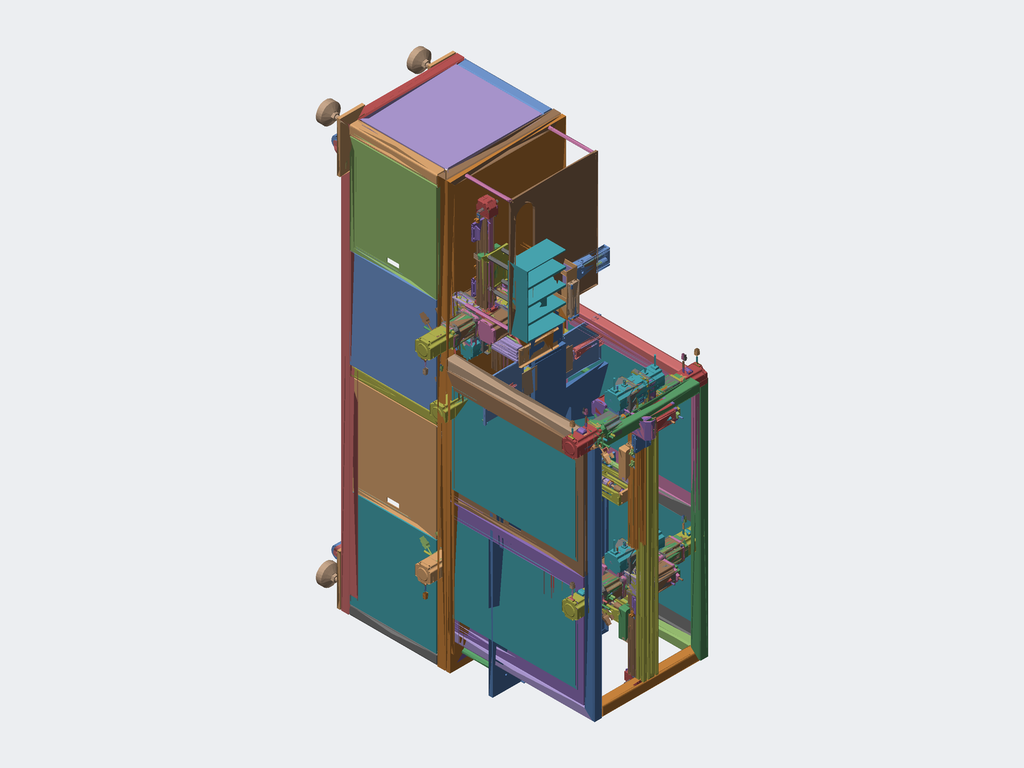Assembly | STEP file | 126 different items | 376 placed
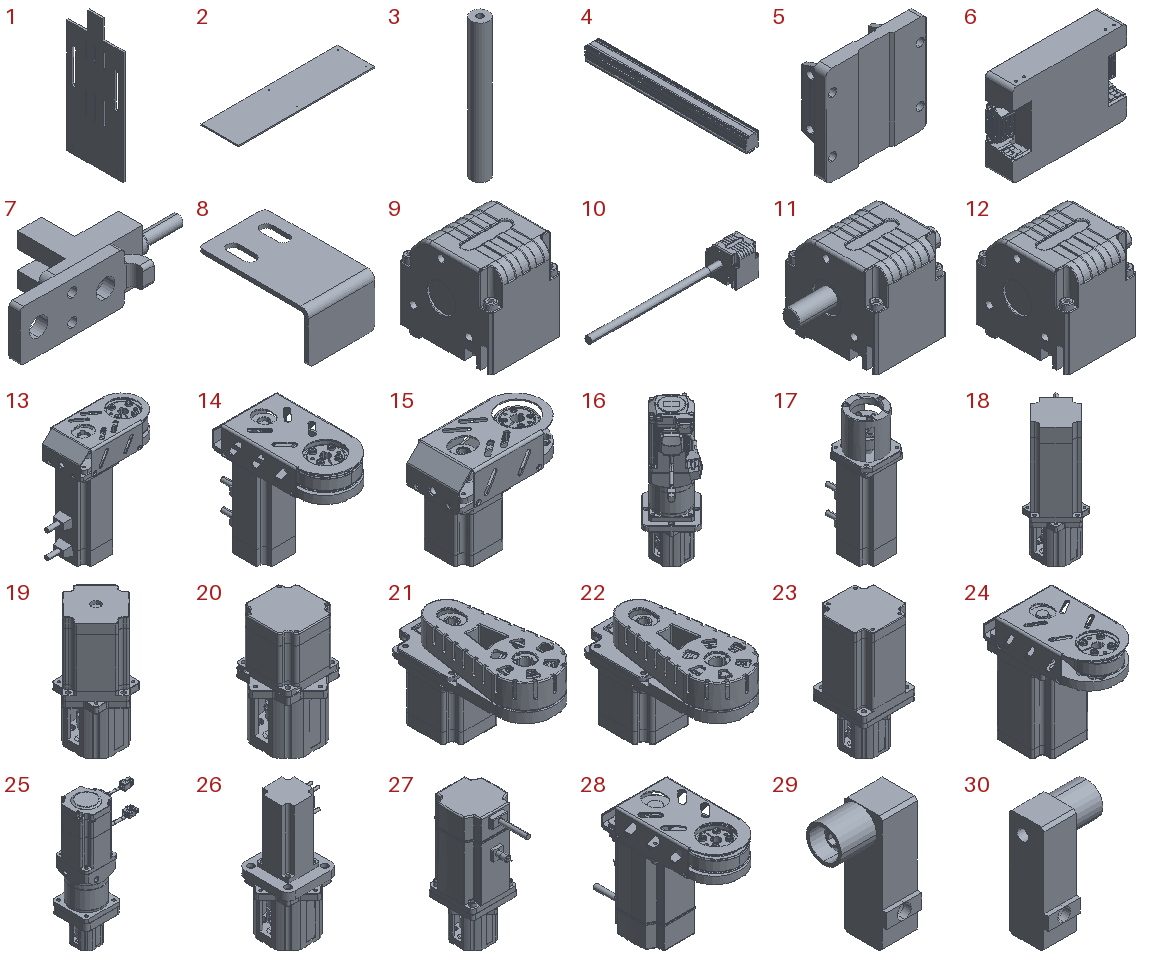Parts list (item | name | quantity | parent item | size | volume):
1 | B1-002 | x1 | in B1-001 | 20.1 x 600 x 1400 mm | 14156369 mm3
2 | B1-003 | x1 | in B1-001 | 2200 x 600 x 20 mm | 26393073 mm3
3 | B1-004 | x4 | in B1-001 | 25 x 25 x 200 mm | 96489 mm3
4 | Copy of 50-2016 profile^K50A-1H20-S(equation-driven)-L | x2 | - | 50 x 565 x 52.45 mm | 1145333 mm3
5 | Copy of 50N support base^K50A-1H20-S(equation-driven)-L | x4 | - | 82 x 32 x 80 mm | 67767 mm3
6 | Copy of K50-4-wheel slider (B version)^K50A-1H20-S(equation-driven)-L | x2 | - | 140 x 34.5 x 102 mm | 434143 mm3
7 | Copy of 50-sensor^K50A-1H20-S(equation-driven)-L | x6 | - | 48.5 x 21.5 x 13.5 mm | 3491 mm3
8 | Copy of K50-004 sensing plate^K50A-1H20-S(equation-driven)-L | x2 | - | 20 x 33 x 15 mm | 1039 mm3
9 | Copy of K50-001A^K50A-1H20-S(equation-driven)-L | x4 | - | 50 x 65 x 67.5 mm | 172642 mm3
10 | Copy of K50-right output shaft^K50A-1H20-S(equation-driven)-L | x2 | - | 325.1 x 65 x 67.5 mm | 214031 mm3
11 | Copy of K50-dual output shaft^K50A-1H20-S(equation-driven)-L | x2 | - | 100.2 x 65 x 67.5 mm | 178596 mm3
12 | Copy of K50-left output shaft^K50A-1H20-S(equation-driven)-L | x2 | - | 75.1 x 65 x 67.5 mm | 175546 mm3
13 | Copy of CZ002-400W side connector 2:1(K60)^K50A-1H20-S(equation-driven)-L | x2 | - | 161.001 x 70 x 175.5 mm | 580294 mm3
14 | Copy of CZ006-400W side connector 3:1(K60)^K50A-1H20-S(equation-driven)-L | x2 | - | 88 x 199.001 x 175.5 mm | 719497 mm3
15 | Copy of C0045-60 side connector 2:1(K60)^K50A-1H20-S(equation-driven)-L | x2 | - | 136.5 x 70 x 107.5 mm | 331047 mm3
16 | Copy of 400W gearbox assembly (universal motor mount plus Q15)^K50A-1H20-S(equation-driven)-L | x2 | - | 131.976 x 164.111 x 242.5 mm | 719537 mm3
17 | Copy of 400W motor assembly (60 motor mount)^K50A-1H20-S(equation-driven)-L | x3 | - | 65 x 95.5 x 200.5 mm | 502014 mm3
18 | Copy of 400W motor assembly (universal motor mount)^K50A-1H20-S(equation-driven)-L | x2 | - | 88.621 x 88.621 x 198.5 mm | 512392 mm3
19 | Copy of 60 motor assembly (universal motor mount)^K50A-1H20-S(equation-driven)-L | x2 | - | 82.65 x 82.65 x 148.5 mm | 366455 mm3
20 | Copy of 57 motor assembly (universal motor mount)^K50A-1H20-S(equation-driven)-L | x2 | - | 82.368 x 82.368 x 117.5 mm | 245014 mm3
21 | Copy of CZ031-57 side connector 2:1(60-60N)^K50A-1H20-S(equation-driven)-L | x2 | - | 60 x 146.25 x 90.3 mm | 270957 mm3
22 | Copy of CZ033-57 side connector 3:1(60-60N)^K50A-1H20-S(equation-driven)-L | x2 | - | 60 x 146.5 x 90.3 mm | 285335 mm3
23 | Copy of 86 motor assembly (universal motor mount)^K50A-1H20-S(equation-driven)-L | x2 | - | 86.045 x 86.045 x 193 mm | 941997 mm3
24 | Copy of CZ020-86 side connector 2:1(K60)^K50A-1H20-S(equation-driven)-L | x2 | - | 88 x 164.5 x 162 mm | 999458 mm3
25 | Copy of 90 gearbox-universal motor mount^K50A-1H20-S(equation-driven)-L | x2 | - | 176.65 x 90 x 314 mm | 1490817 mm3
26 | Copy of 100W motor assembly (universal motor mount)^K50A-1H20-S(equation-driven)-L | x2 | - | 82.368 x 82.368 x 154.9 mm | 253997 mm3
27 | Copy of 750W motor assembly (universal motor mount)^K50A-1H20-S(equation-driven)-L | x2 | - | 82.368 x 139.887 x 214.5 mm | 943398 mm3
28 | Copy of CZ013-750W side connector 2:1(K60)^K50A-1H20-S(equation-driven)-L | x2 | - | 88 x 238.88 x 185 mm | 1086886 mm3
29 | Copy of right hard limit assembly^K50A-1H20-S(equation-driven)-L | x1 | - | 24 x 15.5 x 40 mm | 6072 mm3
30 | Copy of left hard limit assembly^K50A-1H20-S(equation-driven)-L | x1 | - | 24 x 15.5 x 40 mm | 6072 mm3
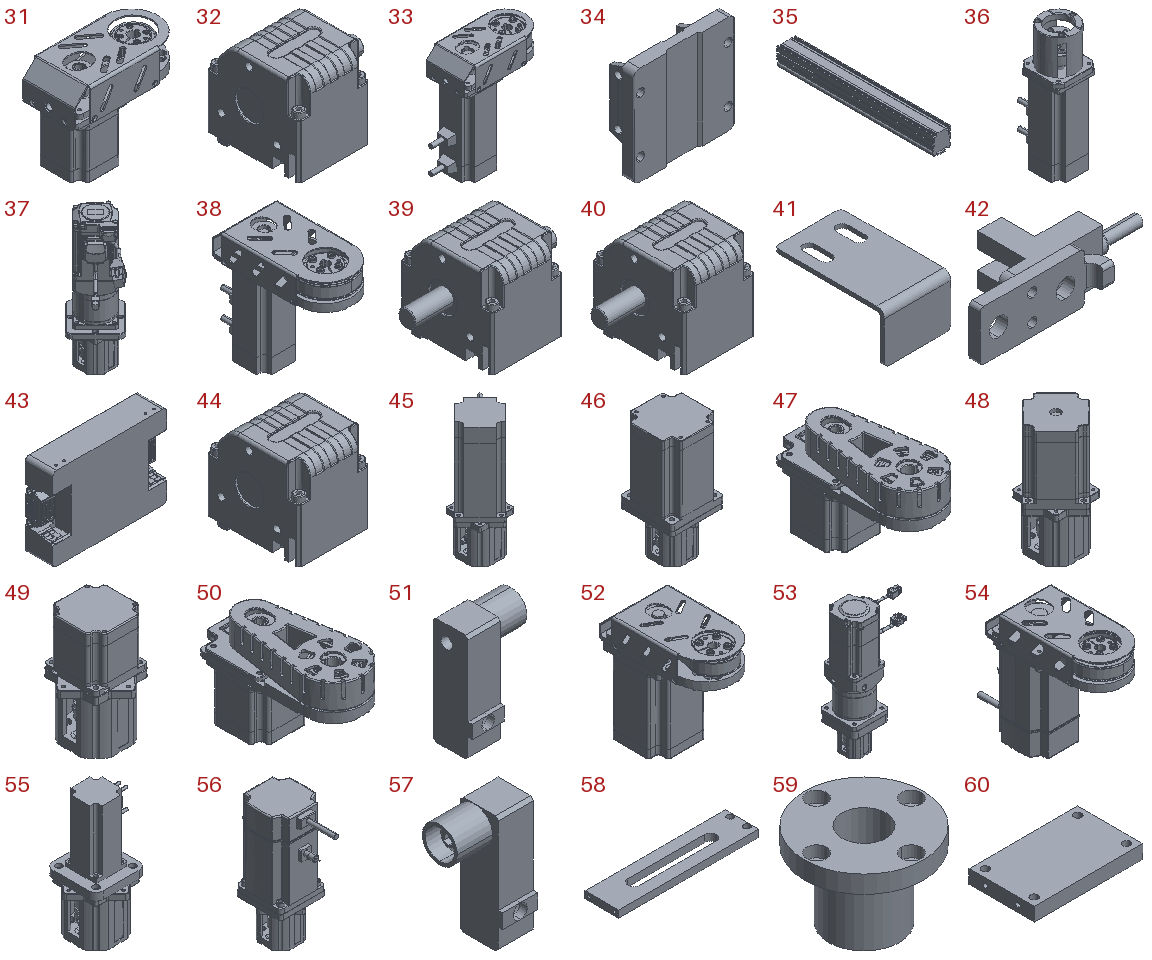31 | Copy of C0045-60 side connector 2:1(K60)^K50A-1H20-S(equation-driven)-L0 | x6 | - | 136.5 x 70 x 107.5 mm | 331047 mm3
32 | Copy of K50-left output shaft^K50A-1H20-S(equation-driven)-L0 | x6 | - | 75.1 x 65 x 67.5 mm | 175546 mm3
33 | Copy of CZ002-400W side connector 2:1(K60)^K50A-1H20-S(equation-driven)-L0 | x6 | - | 161.001 x 70 x 175.5 mm | 580294 mm3
34 | Copy of 50N support base^K50A-1H20-S(equation-driven)-L0 | x6 | - | 82 x 32 x 80 mm | 67767 mm3
35 | Copy of 50-2016 profile^K50A-1H20-S(equation-driven)-L0 | x3 | - | 50 x 415 x 52.45 mm | 841262 mm3
36 | Copy of 400W motor assembly (60 motor mount)^K50A-1H20-S(equation-driven)-L0 | x6 | - | 65 x 95.5 x 200.5 mm | 502014 mm3
37 | Copy of 400W gearbox assembly (universal motor mount plus Q15)^K50A-1H20-S(equation-driven)-L0 | x6 | - | 131.976 x 164.111 x 242.5 mm | 719537 mm3
38 | Copy of CZ006-400W side connector 3:1(K60)^K50A-1H20-S(equation-driven)-L0 | x6 | - | 88 x 199.001 x 175.5 mm | 672015 mm3
39 | Copy of K50-dual output shaft^K50A-1H20-S(equation-driven)-L0 | x6 | - | 100.2 x 65 x 67.5 mm | 178596 mm3
40 | Copy of K50-right output shaft^K50A-1H20-S(equation-driven)-L0 | x6 | - | 75.1 x 65 x 67.5 mm | 175546 mm3
41 | Copy of K50-004 sensing plate^K50A-1H20-S(equation-driven)-L0 | x3 | - | 20 x 33 x 15 mm | 1039 mm3
42 | Copy of 50-Sensor^K50A-1H20-S(equation-driven)-L0 | x9 | - | 48.5 x 21.5 x 13.5 mm | 3491 mm3
43 | Copy of K50-4-wheel slider (B version)^K50A-1H20-S(equation-driven)-L0 | x3 | - | 140 x 34.5 x 102 mm | 434143 mm3
44 | Copy of K50-001A^K50A-1H20-S(equation-driven)-L0 | x6 | - | 50 x 65 x 67.5 mm | 172642 mm3
45 | Copy of 400W motor assembly (universal motor mount)^K50A-1H20-S(equation-driven)-L0 | x6 | - | 88.621 x 88.621 x 198.5 mm | 512392 mm3
46 | Copy of 86 motor assembly (universal motor mount)^K50A-1H20-S(equation-driven)-L0 | x6 | - | 86.045 x 86.045 x 193 mm | 941997 mm3
47 | Copy of CZ033-57 side connector 3:1(60-60N)^K50A-1H20-S(equation-driven)-L0 | x6 | - | 60 x 146.5 x 90.3 mm | 285335 mm3
48 | Copy of 60 motor assembly (universal motor mount)^K50A-1H20-S(equation-driven)-L0 | x6 | - | 82.65 x 82.65 x 148.5 mm | 366455 mm3
49 | Copy of 57 motor assembly (universal motor mount)^K50A-1H20-S(equation-driven)-L0 | x6 | - | 82.368 x 82.368 x 117.5 mm | 245014 mm3
50 | Copy of CZ031-57 side connector 2:1(60-60N)^K50A-1H20-S(equation-driven)-L0 | x6 | - | 60 x 146.25 x 90.3 mm | 270957 mm3
51 | Copy of left hard limit assembly^K50A-1H20-S(equation-driven)-L0 | x3 | - | 24 x 15.5 x 40 mm | 6072 mm3
52 | Copy of CZ020-86 side connector 2:1(K60)^K50A-1H20-S(equation-driven)-L0 | x6 | - | 88 x 164.5 x 162 mm | 999458 mm3
53 | Copy of 90 gearbox-universal motor mount^K50A-1H20-S(equation-driven)-L0 | x6 | - | 176.65 x 90 x 314 mm | 1490817 mm3
54 | Copy of CZ013-750W side connector 2:1(K60)^K50A-1H20-S(equation-driven)-L0 | x6 | - | 88 x 238.88 x 185 mm | 1086886 mm3
55 | Copy of 100W motor assembly (universal motor mount)^K50A-1H20-S(equation-driven)-L0 | x6 | - | 82.368 x 82.368 x 154.9 mm | 253997 mm3
56 | Copy of 750W motor assembly (universal motor mount)^K50A-1H20-S(equation-driven)-L0 | x6 | - | 82.368 x 139.887 x 214.5 mm | 943398 mm3
57 | Copy of right hard limit assembly^K50A-1H20-S(equation-driven)-L0 | x3 | - | 24 x 15.5 x 40 mm | 6072 mm3
58 | B1-006 | x4 | in 1 | 200 x 48 x 10 mm | 75143 mm3
59 | LMF01-d20-steel outer graphite inner- | x4 | in 1 | 54 x 54 x 38 mm | 28938 mm3
60 | B1-005 | x2 | in 1 | 80 x 48 x 10 mm | 37093 mm3
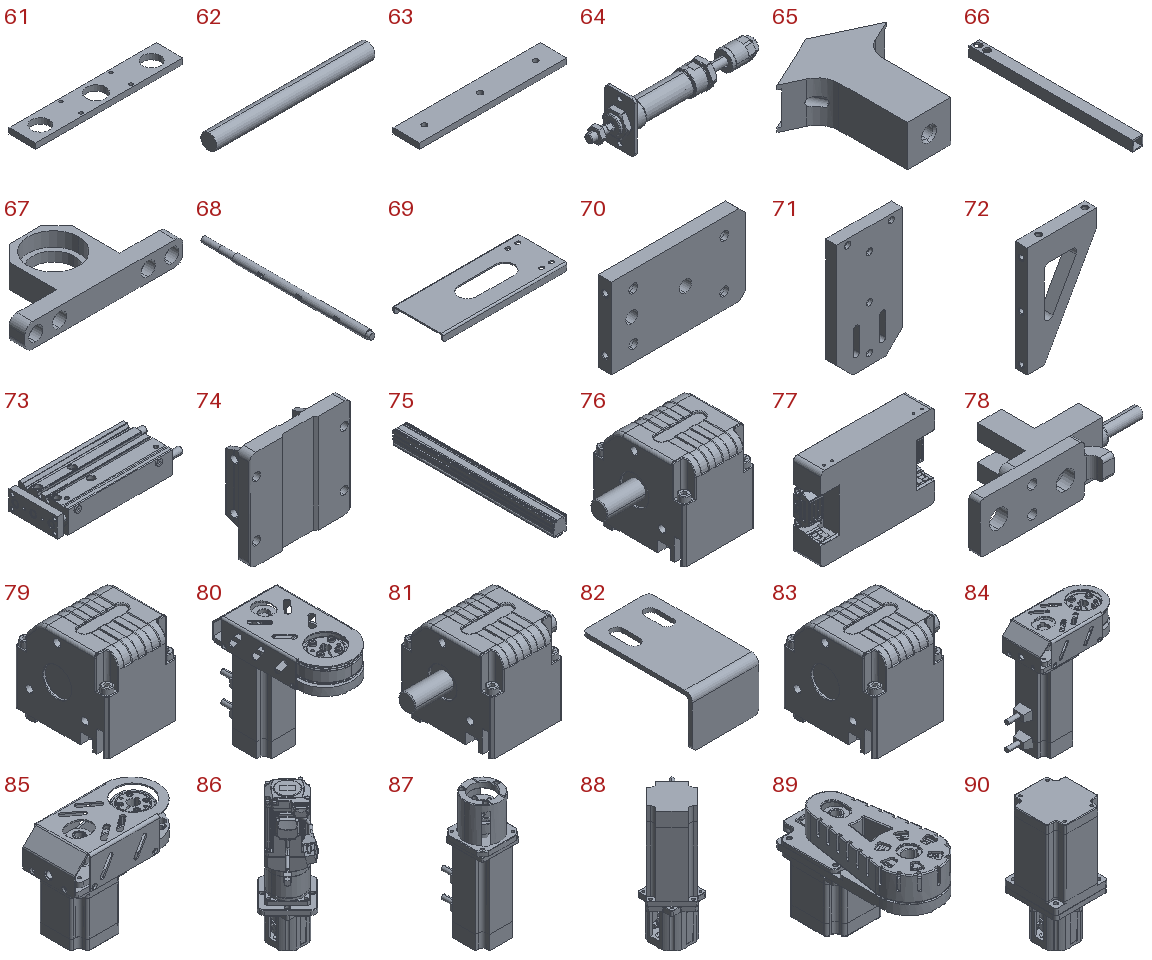61 | B1-007 | x2 | in 1 | 265 x 48 x 10 mm | 99587 mm3
62 | B1-009 | x4 | in 1 | 200 x 20 x 20 mm | 62632 mm3
63 | B1-008 | x2 | in 1 | 265 x 48 x 10 mm | 125461 mm3
64 | - | x2 | in 1 | 211 x 38 x 64 mm | 90003 mm3
65 | B1-013 | x6 | in 2, 3 | 40 x 45 x 15 mm | 11495 mm3
66 | B1-010 | x4 | in 2, 3 | 12 x 190 x 12 mm | 11800 mm3
67 | B1-011 | x4 | in 2, 3 | 100 x 50 x 15 mm | 24955 mm3
68 | B1-012 | x2 | in 2, 3 | 20 x 445 x 20 mm | 123230 mm3
69 | B1-017 | x3 | in 60, 58 | 200 x 80 x 12 mm | 34069 mm3
70 | B1-014 | x3 | in 60, 58 | 100 x 10 x 60 mm | 55350 mm3
71 | B1-015 | x3 | in 60, 58 | 60 x 10 x 110 mm | 58492 mm3
72 | B1-016 | x3 | in 60, 58 | 60 x 10 x 95 mm | 30263 mm3
73 | TCL16x100S_0_ | x3 | in 60, 58 | 165 x 66.1 x 30 mm | 211792 mm3
74 | Copy of 50N support base^K50A-1H20-S(equation-driven)-L1 | x2 | - | 82 x 32 x 80 mm | 67767 mm3
75 | Copy of 50-2016 profile^K50A-1H20-S(equation-driven)-L1 | x1 | - | 50 x 565 x 52.45 mm | 1145333 mm3
76 | Copy of K50-right output shaft^K50A-1H20-S(equation-driven)-L1 | x2 | - | 75.1 x 65 x 67.5 mm | 175546 mm3
77 | Copy of K50-4-wheel slider (B version)^K50A-1H20-S(equation-driven)-L1 | x1 | - | 140 x 34.5 x 102 mm | 434143 mm3
78 | Copy of 50-sensor^K50A-1H20-S(equation-driven)-L1 | x3 | - | 48.5 x 21.5 x 13.5 mm | 3491 mm3
79 | Copy of K50-001A^K50A-1H20-S(equation-driven)-L1 | x2 | - | 50 x 65 x 67.5 mm | 172642 mm3
80 | Copy of CZ006-400W side connector 3:1(K60)^K50A-1H20-S(equation-driven)-L1 | x2 | - | 88 x 199.001 x 175.5 mm | 672015 mm3
81 | Copy of K50-dual output shaft^K50A-1H20-S(equation-driven)-L1 | x2 | - | 100.2 x 65 x 67.5 mm | 178596 mm3
82 | Copy of K50-004 sensing plate^K50A-1H20-S(equation-driven)-L1 | x1 | - | 20 x 33 x 15 mm | 1039 mm3
83 | Copy of K50-left output shaft^K50A-1H20-S(equation-driven)-L1 | x2 | - | 75.1 x 65 x 67.5 mm | 175546 mm3
84 | Copy of CZ002-400W side connector 2:1(K60)^K50A-1H20-S(equation-driven)-L1 | x2 | - | 161.001 x 70 x 175.5 mm | 580294 mm3
85 | Copy of C0045-60 side connector 2:1(K60)^K50A-1H20-S(equation-driven)-L1 | x2 | - | 136.5 x 70 x 107.5 mm | 331047 mm3
86 | Copy of 400W gearbox assembly (universal motor mount plus Q15)^K50A-1H20-S(equation-driven)-L1 | x2 | - | 131.976 x 164.111 x 242.5 mm | 719537 mm3
87 | Copy of 400W motor assembly (60 motor mount)^K50A-1H20-S(equation-driven)-L1 | x2 | - | 65 x 95.5 x 200.5 mm | 502014 mm3
88 | Copy of 400W motor assembly (universal motor mount)^K50A-1H20-S(equation-driven)-L1 | x2 | - | 88.621 x 88.621 x 198.5 mm | 512392 mm3
89 | Copy of CZ033-57 side connector 3:1(60-60N)^K50A-1H20-S(equation-driven)-L1 | x2 | - | 60 x 146.5 x 90.3 mm | 285335 mm3
90 | Copy of 86 motor assembly (universal motor mount)^K50A-1H20-S(equation-driven)-L1 | x2 | - | 86.045 x 86.045 x 193 mm | 941997 mm3
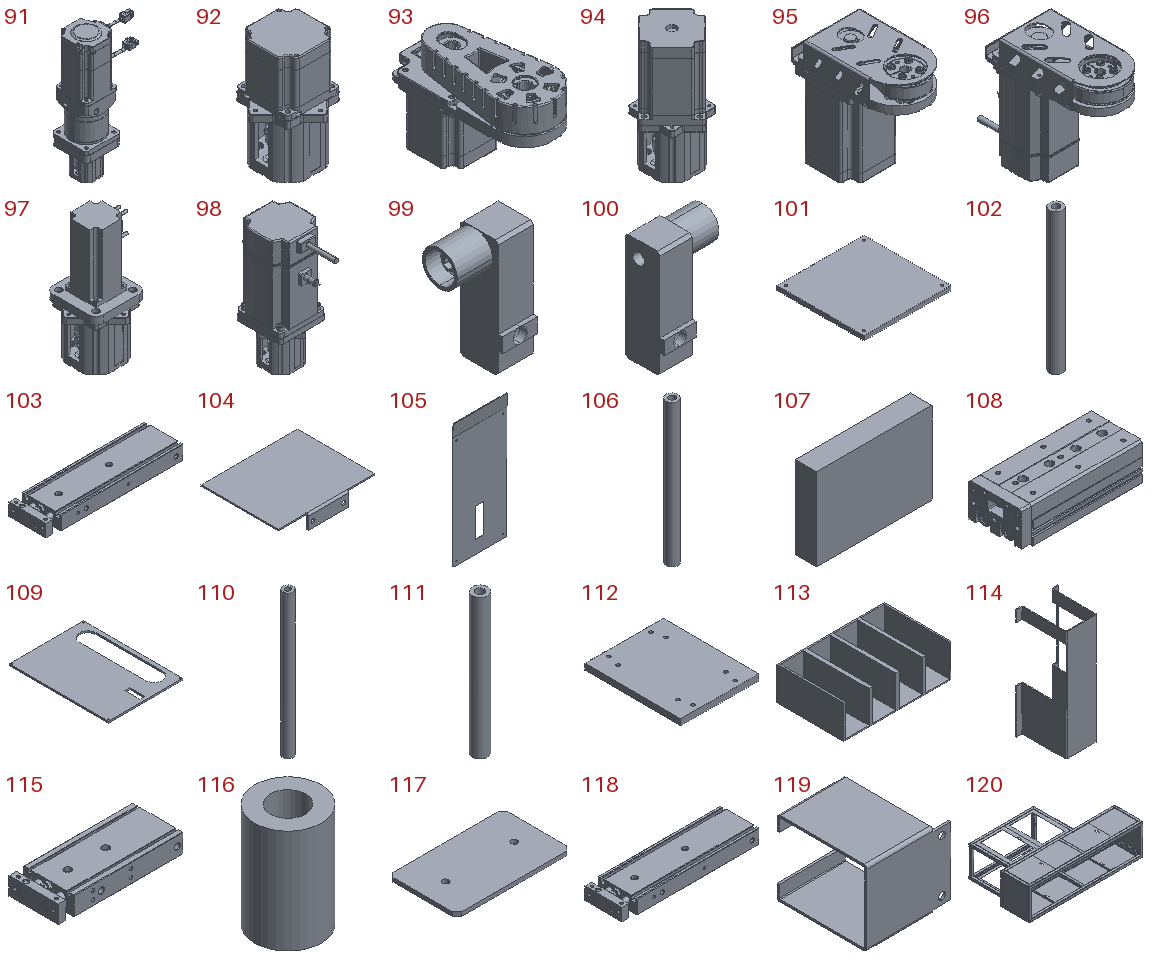91 | Copy of 90 gearbox-universal motor mount^K50A-1H20-S(equation-driven)-L1 | x2 | - | 176.65 x 90 x 314 mm | 1490817 mm3
92 | Copy of 57 motor assembly (universal motor mount)^K50A-1H20-S(equation-driven)-L1 | x2 | - | 82.368 x 82.368 x 117.5 mm | 245014 mm3
93 | Copy of CZ031-57 side connector 2:1(60-60N)^K50A-1H20-S(equation-driven)-L1 | x2 | - | 60 x 146.25 x 90.3 mm | 270957 mm3
94 | Copy of 60 motor assembly (universal motor mount)^K50A-1H20-S(equation-driven)-L1 | x2 | - | 82.65 x 82.65 x 148.5 mm | 366455 mm3
95 | Copy of CZ020-86 side connector 2:1(K60)^K50A-1H20-S(equation-driven)-L1 | x2 | - | 88 x 164.5 x 162 mm | 999458 mm3
96 | Copy of CZ013-750W side connector 2:1(K60)^K50A-1H20-S(equation-driven)-L1 | x2 | - | 88 x 238.88 x 185 mm | 1086886 mm3
97 | Copy of 100W motor assembly (universal motor mount)^K50A-1H20-S(equation-driven)-L1 | x2 | - | 82.368 x 82.368 x 154.9 mm | 253997 mm3
98 | Copy of 750W motor assembly (universal motor mount)^K50A-1H20-S(equation-driven)-L1 | x2 | - | 82.368 x 139.887 x 214.5 mm | 943398 mm3
99 | Copy of right hard limit assembly^K50A-1H20-S(equation-driven)-L1 | x1 | - | 24 x 15.5 x 40 mm | 6072 mm3
100 | Copy of left hard limit assembly^K50A-1H20-S(equation-driven)-L1 | x1 | - | 24 x 15.5 x 40 mm | 6072 mm3
101 | B1-018 | x2 | in B1-001 | 200 x 200 x 10 mm | 399050 mm3
102 | B1-019 | x8 | in B1-001 | 16 x 16 x 172 mm | 32897 mm3
103 | - | x2 | in B1-001 | 162 x 46 x 17 mm | 100812 mm3
104 | B1-020 | x2 | in B1-001 | 110 x 90 x 16 mm | 15572 mm3
105 | B1-021 | x1 | in B1-001 | 170 x 4.986 x 389.979 mm | 95964 mm3
106 | B1-022 | x3 | in B1-001 | 16 x 16 x 196.5 mm | 37823 mm3
107 | B1-023 | x1 | in B1-001 | 120 x 22 x 85 mm | 224378 mm3
108 | - | x1 | in B1-001 | 161 x 70 x 50 mm | 433153 mm3
109 | B1-024 | x1 | in B1-001 | 450 x 600 x 10 mm | 2193510 mm3
110 | B1-025 | x4 | in B1-001 | 16 x 16 x 230 mm | 44559 mm3
111 | B1-027 | x4 | in 61 | 16 x 16 x 145 mm | 27469 mm3
112 | B1-026 | x2 | in 61 | 130 x 160 x 10 mm | 206099 mm3
113 | B1-028 | x1 | in B1-001 | 320 x 200 x 100 mm | 1158400 mm3
114 | B1-029 | x1 | in B1-001 | 77 x 81.5 x 200 mm | 43403 mm3
115 | - | x1 | in B1-001 | 196 x 80 x 30 mm | 343532 mm3
116 | B1-030 | x2 | in B1-001 | 16 x 16 x 25 mm | 3608 mm3
117 | B1-031 | x1 | in B1-001 | 100 x 60 x 3.5 mm | 20722 mm3
118 | - | x1 | in B1-001 | 162 x 46 x 17 mm | 100309 mm3
119 | B1-032 | x1 | in B1-001 | 56 x 60 x 50 mm | 12765 mm3
120 | - | x1 | in B1-001 | 2200 x 1312 x 600 mm | 17312645 mm3
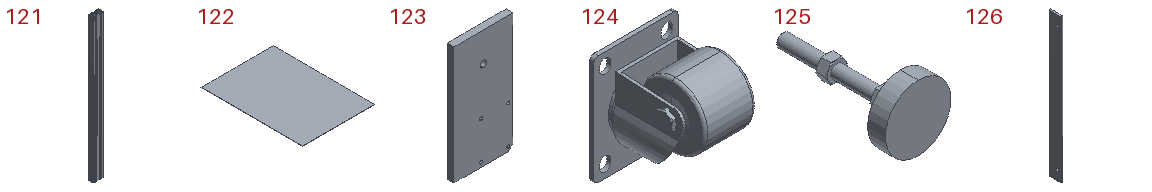121 | LE-8-4080W-S-OO_LE0912125351 | x1 | in B1-001 | 80 x 40 x 1150 mm | 1377772 mm3
122 | B1-033 | x4 | in B1-001 | 460 x 650 x 1.5 mm | 448500 mm3
123 | PN_0001_default<by machining> | x4 | in B1-001 | 130 x 15 x 260 mm | 501762 mm3
124 | CGL01-D63- | x4 | in B1-001 | 82 x 96 x 111.5 mm | 244829 mm3
125 | WAM05-D100-M16-L100- | x4 | in B1-001 | 100 x 207 x 100 mm | 345017 mm3
126 | B1-034 | x1 | in B1-001 | 3.5 x 25 x 300 mm | 26084 mm3
Placements (level | parent | child | x y z in mm | rotation matrix by rows), first 211 of 388 lines:
1 | B1-001 | B1-002 | -17.166 -47.036 1200.0 | 1 0 0 0 1 0 0 0 1
1 | B1-001 | B1-003 | -237.166 -47.036 1550.0 | 0 0 1 0 1 0 -1 0 0
1 | B1-001 | B1-004 | -127.166 182.964 520.0 | 0 0 -1 0 1 0 1 0 -0
1 | B1-001 | B1-004 | -127.166 -277.036 520.0 | 0 0 -1 0 1 0 1 0 -0
1 | B1-001 | B1-004 | -127.166 182.964 1630.0 | 0 0 -1 0 1 0 1 0 -0
1 | B1-001 | B1-004 | -127.166 -277.036 1630.0 | 0 0 -1 0 1 0 1 0 -0
1 | B1-001 | subassembly 2 | -217.166 -197.036 1040.0 | 0 1 0 -1 0 0 0 0 1
2 | subassembly 2 | Copy of 50-2016 profile^K50A-1H20-S(equation-driven)-L | -0.0 -0.0 -0.0 | 1 0 0 0 0 -1 0 1 -0
2 | subassembly 2 | Copy of 50N support base^K50A-1H20-S(equation-driven)-L | -0.0 -10.0 475.0 | 1 0 0 0 1 0 0 0 1
2 | subassembly 2 | Copy of K50-4-wheel slider (B version)^K50A-1H20-S(equation-driven)-L | 142.0 50.55 195.197 | 0 0 -1 0 1 0 1 0 0
2 | subassembly 2 | Copy of 50-sensor^K50A-1H20-S(equation-driven)-L | 24.949 47.3 540.944 | 0 1 0 0 0 -1 -1 0 0
2 | subassembly 2 | Copy of K50-004 sensing plate^K50A-1H20-S(equation-driven)-L | 52.2 30.2 243.357 | 0 0 1 0 1 0 -1 0 -0
2 | subassembly 2 | Copy of 50-sensor^K50A-1H20-S(equation-driven)-L | 24.949 47.3 130.144 | 0 1 0 0 0 -1 -1 0 0
2 | subassembly 2 | Copy of 50-sensor^K50A-1H20-S(equation-driven)-L | 24.949 47.3 181.144 | 0 1 0 0 0 -1 -1 0 0
2 | subassembly 2 | Copy of K50-001A^K50A-1H20-S(equation-driven)-L | -1.386 27.562 115.0 | 1 0 0 0 1 0 0 0 1
2 | subassembly 2 | Copy of K50-001A^K50A-1H20-S(equation-driven)-L | 1.386 27.562 450.0 | -1 0 0 0 1 0 0 0 -1
2 | subassembly 2 | Copy of K50-right output shaft^K50A-1H20-S(equation-driven)-L | 1.386 27.562 450.0 | -1 0 0 0 1 0 0 0 -1
2 | subassembly 2 | Copy of K50-right output shaft^K50A-1H20-S(equation-driven)-L | -1.386 27.562 115.0 | 1 0 0 0 1 0 0 0 1
2 | subassembly 2 | Copy of K50-dual output shaft^K50A-1H20-S(equation-driven)-L | -1.386 27.562 115.0 | 1 0 0 0 1 0 0 0 1
2 | subassembly 2 | Copy of K50-dual output shaft^K50A-1H20-S(equation-driven)-L | 1.386 27.562 450.0 | -1 0 0 0 1 0 0 0 -1
2 | subassembly 2 | Copy of K50-left output shaft^K50A-1H20-S(equation-driven)-L | -1.386 27.562 115.0 | 1 0 0 0 1 0 0 0 1
2 | subassembly 2 | Copy of K50-left output shaft^K50A-1H20-S(equation-driven)-L | 1.386 27.562 450.0 | -1 0 0 0 1 0 0 0 -1
2 | subassembly 2 | Copy of 50N support base^K50A-1H20-S(equation-driven)-L | -0.0 -10.0 79.0 | 1 0 0 0 1 0 0 0 1
2 | subassembly 2 | Copy of CZ002-400W side connector 2:1(K60)^K50A-1H20-S(equation-driven)-L | -137.949 50.063 -41.164 | 0 0 1 -1 0 0 0 -1 0
2 | subassembly 2 | Copy of CZ006-400W side connector 3:1(K60)^K50A-1H20-S(equation-driven)-L | -139.254 -53.524 5.303 | 0 0 1 0 -1 0 1 0 -0
2 | subassembly 2 | Copy of CZ006-400W side connector 3:1(K60)^K50A-1H20-S(equation-driven)-L | 139.254 70.303 -118.524 | 0 0 -1 1 0 0 0 -1 -0
2 | subassembly 2 | Copy of CZ002-400W side connector 2:1(K60)^K50A-1H20-S(equation-driven)-L | 137.949 46.164 -45.063 | 0 0 -1 0 1 0 1 0 0
2 | subassembly 2 | Copy of C0045-60 side connector 2:1(K60)^K50A-1H20-S(equation-driven)-L | -137.949 50.063 -41.164 | 0 0 1 -1 0 0 0 -1 0
2 | subassembly 2 | Copy of C0045-60 side connector 2:1(K60)^K50A-1H20-S(equation-driven)-L | 137.949 46.164 -45.063 | 0 0 -1 0 1 0 1 0 -0
2 | subassembly 2 | Copy of 400W gearbox assembly (universal motor mount plus Q15)^K50A-1H20-S(equation-driven)-L | 28.0 35.0 -30.0 | 0 0 1 0 1 0 -1 0 0
2 | subassembly 2 | Copy of 400W motor assembly (60 motor mount)^K50A-1H20-S(equation-driven)-L | 58.836 40.482 14.041 | 0 0 -1 0 -1 0 -1 0 0
2 | subassembly 2 | Copy of 400W motor assembly (universal motor mount)^K50A-1H20-S(equation-driven)-L | -25.868 28.042 -17.555 | 0 0 1 0 1 0 -1 0 0
2 | subassembly 2 | Copy of 400W gearbox assembly (universal motor mount plus Q15)^K50A-1H20-S(equation-driven)-L | -28.0 35.0 -30.0 | 0 0 -1 0 -1 0 -1 0 -0
2 | subassembly 2 | Copy of 400W motor assembly (universal motor mount)^K50A-1H20-S(equation-driven)-L | 25.868 41.958 -17.555 | 0 0 -1 0 -1 0 -1 0 -0
2 | subassembly 2 | Copy of 400W motor assembly (60 motor mount)^K50A-1H20-S(equation-driven)-L | -58.836 29.518 14.041 | 0 0 1 0 1 0 -1 0 -0
2 | subassembly 2 | Copy of 60 motor assembly (universal motor mount)^K50A-1H20-S(equation-driven)-L | 25.868 42.444 -32.04 | 0 0 -1 0 -1 0 -1 0 -0
2 | subassembly 2 | Copy of 60 motor assembly (universal motor mount)^K50A-1H20-S(equation-driven)-L | -25.868 27.556 -32.04 | 0 0 1 0 1 0 -1 0 0
2 | subassembly 2 | Copy of 57 motor assembly (universal motor mount)^K50A-1H20-S(equation-driven)-L | -25.867 39.661 -53.676 | 0 0 1 0 1 0 -1 0 0
2 | subassembly 2 | Copy of CZ031-57 side connector 2:1(60-60N)^K50A-1H20-S(equation-driven)-L | -107.0 78.623 -31.684 | 0 0 1 0 1 0 -1 0 0
2 | subassembly 2 | Copy of CZ033-57 side connector 3:1(60-60N)^K50A-1H20-S(equation-driven)-L | -107.0 78.623 -31.684 | 0 0 1 0 1 0 -1 0 -0
2 | subassembly 2 | Copy of CZ033-57 side connector 3:1(60-60N)^K50A-1H20-S(equation-driven)-L | 107.0 36.684 -73.623 | 0 0 -1 1 0 0 0 -1 -0
2 | subassembly 2 | Copy of CZ031-57 side connector 2:1(60-60N)^K50A-1H20-S(equation-driven)-L | 107.0 36.684 -73.623 | 0 0 -1 1 0 0 0 -1 -0
2 | subassembly 2 | Copy of 57 motor assembly (universal motor mount)^K50A-1H20-S(equation-driven)-L | 25.867 30.339 -53.676 | 0 0 -1 0 -1 0 -1 0 -0
2 | subassembly 2 | Copy of 86 motor assembly (universal motor mount)^K50A-1H20-S(equation-driven)-L | -25.868 26.685 -28.19 | 0 0 1 0 1 0 -1 0 0
2 | subassembly 2 | Copy of 86 motor assembly (universal motor mount)^K50A-1H20-S(equation-driven)-L | 25.868 43.315 -28.19 | 0 0 -1 0 -1 0 -1 0 -0
2 | subassembly 2 | Copy of CZ020-86 side connector 2:1(K60)^K50A-1H20-S(equation-driven)-L | -131.645 -38.755 -4.508 | 0 0 1 0 -1 0 1 0 0
2 | subassembly 2 | Copy of CZ020-86 side connector 2:1(K60)^K50A-1H20-S(equation-driven)-L | 131.645 108.755 -4.508 | 0 0 -1 0 1 0 1 0 0
2 | subassembly 2 | Copy of 90 gearbox-universal motor mount^K50A-1H20-S(equation-driven)-L | 4.902 63.56 -46.01 | 0 0 1 0 1 0 -1 0 0
2 | subassembly 2 | Copy of 90 gearbox-universal motor mount^K50A-1H20-S(equation-driven)-L | -4.902 6.44 -46.01 | 0 0 -1 0 -1 0 -1 0 -0
2 | subassembly 2 | Copy of 100W motor assembly (universal motor mount)^K50A-1H20-S(equation-driven)-L | -25.868 30.418 -8.844 | 0 0 1 0 1 0 -1 0 0
2 | subassembly 2 | Copy of 100W motor assembly (universal motor mount)^K50A-1H20-S(equation-driven)-L | 25.868 39.582 -8.844 | 0 0 -1 0 -1 0 -1 0 -0
2 | subassembly 2 | Copy of 750W motor assembly (universal motor mount)^K50A-1H20-S(equation-driven)-L | -25.868 36.188 -29.887 | 0 0 1 0 1 0 -1 0 0
2 | subassembly 2 | Copy of CZ013-750W side connector 2:1(K60)^K50A-1H20-S(equation-driven)-L | -83.709 -0.3027 -12.512 | 0 0 1 -1 0 0 0 -1 0
2 | subassembly 2 | Copy of CZ013-750W side connector 2:1(K60)^K50A-1H20-S(equation-driven)-L | 83.709 70.303 -12.512 | 0 0 -1 1 0 0 0 -1 -0
2 | subassembly 2 | Copy of 750W motor assembly (universal motor mount)^K50A-1H20-S(equation-driven)-L | 25.868 33.812 -29.887 | 0 0 -1 0 -1 0 -1 0 -0
2 | subassembly 2 | Copy of right hard limit assembly^K50A-1H20-S(equation-driven)-L | -31.412 -15.95 14.722 | 0 -1 0 0 0 1 -1 0 0
2 | subassembly 2 | Copy of left hard limit assembly^K50A-1H20-S(equation-driven)-L | 31.913 -15.95 20.751 | 0 1 0 0 0 1 1 0 -0
2 | subassembly 2 | Copy of 50N support base^K50A-1H20-S(equation-driven)-L | -300.0 -10.0 79.0 | 1 0 0 0 1 0 0 0 1
2 | subassembly 2 | Copy of K50-004 sensing plate^K50A-1H20-S(equation-driven)-L | -247.8 30.2 243.357 | 0 0 1 0 1 0 -1 0 -0
2 | subassembly 2 | Copy of K50-001A^K50A-1H20-S(equation-driven)-L | -301.386 27.562 115.0 | 1 0 0 0 1 0 0 0 1
2 | subassembly 2 | Copy of 50-sensor^K50A-1H20-S(equation-driven)-L | -275.051 47.3 130.144 | 0 1 0 0 0 -1 -1 0 0
2 | subassembly 2 | Copy of 50-2016 profile^K50A-1H20-S(equation-driven)-L | -300.0 -0.0 0.0 | 1 0 0 0 0 -1 0 1 -0
2 | subassembly 2 | Copy of 50-sensor^K50A-1H20-S(equation-driven)-L | -275.051 47.3 540.944 | 0 1 0 0 0 -1 -1 0 0
2 | subassembly 2 | Copy of 50N support base^K50A-1H20-S(equation-driven)-L | -300.0 -10.0 475.0 | 1 0 0 0 1 0 0 0 1
2 | subassembly 2 | Copy of K50-4-wheel slider (B version)^K50A-1H20-S(equation-driven)-L | -158.0 50.55 195.197 | 0 0 -1 0 1 0 1 0 0
2 | subassembly 2 | Copy of 50-sensor^K50A-1H20-S(equation-driven)-L | -275.051 47.3 181.144 | 0 1 0 0 0 -1 -1 0 0
2 | subassembly 2 | Copy of K50-001A^K50A-1H20-S(equation-driven)-L | -298.614 27.562 450.0 | -1 0 0 0 1 0 0 0 -1
2 | subassembly 2 | Copy of 400W motor assembly (60 motor mount)^K50A-1H20-S(equation-driven)-L | -358.836 29.518 14.041 | 0 0 1 0 1 0 -1 0 -0
1 | B1-001 | subassembly 2 | 464.127 -47.036 1050.0 | 0 -1 0 -1 0 0 0 0 -1
2 | subassembly 2 | Copy of C0045-60 side connector 2:1(K60)^K50A-1H20-S(equation-driven)-L0 | -137.949 50.063 -41.164 | 0 0 1 -1 0 0 0 -1 0
2 | subassembly 2 | Copy of K50-left output shaft^K50A-1H20-S(equation-driven)-L0 | -1.386 27.562 -35.0 | 1 0 0 0 1 0 0 0 1
2 | subassembly 2 | Copy of K50-left output shaft^K50A-1H20-S(equation-driven)-L0 | 1.386 27.562 450.0 | -1 0 0 0 1 0 0 0 -1
2 | subassembly 2 | Copy of CZ002-400W side connector 2:1(K60)^K50A-1H20-S(equation-driven)-L0 | -137.949 50.063 -41.164 | 0 0 1 -1 0 0 0 -1 0
2 | subassembly 2 | Copy of 50N support base^K50A-1H20-S(equation-driven)-L0 | -0.0 -10.0 79.0 | 1 0 0 0 1 0 0 0 1
2 | subassembly 2 | Copy of 50-2016 profile^K50A-1H20-S(equation-driven)-L0 | -0.0 -0.0 -0.0 | 1 0 0 0 0 -1 0 1 0
2 | subassembly 2 | Copy of 400W motor assembly (60 motor mount)^K50A-1H20-S(equation-driven)-L0 | 58.836 40.482 14.041 | 0 0 -1 0 -1 0 -1 0 0
2 | subassembly 2 | Copy of 400W gearbox assembly (universal motor mount plus Q15)^K50A-1H20-S(equation-driven)-L0 | 28.0 35.0 -30.0 | 0 0 1 0 1 0 -1 0 0
2 | subassembly 2 | Copy of CZ006-400W side connector 3:1(K60)^K50A-1H20-S(equation-driven)-L0 | -139.254 -53.524 5.303 | 0 0 1 0 -1 0 1 0 -0
2 | subassembly 2 | Copy of CZ006-400W side connector 3:1(K60)^K50A-1H20-S(equation-driven)-L0 | 139.254 70.303 -118.524 | 0 0 -1 1 0 0 0 -1 -0
2 | subassembly 2 | Copy of CZ002-400W side connector 2:1(K60)^K50A-1H20-S(equation-driven)-L0 | 137.949 46.164 -45.063 | 0 0 -1 0 1 0 1 0 0
2 | subassembly 2 | Copy of K50-dual output shaft^K50A-1H20-S(equation-driven)-L0 | 1.386 27.562 450.0 | -1 0 0 0 1 0 0 0 -1
2 | subassembly 2 | Copy of K50-right output shaft^K50A-1H20-S(equation-driven)-L0 | -1.386 27.562 -35.0 | 1 0 0 0 1 0 0 0 1
2 | subassembly 2 | Copy of K50-dual output shaft^K50A-1H20-S(equation-driven)-L0 | -1.386 27.562 -35.0 | 1 0 0 0 1 0 0 0 1
2 | subassembly 2 | Copy of K50-004 sensing plate^K50A-1H20-S(equation-driven)-L0 | 52.2 30.2 241.072 | 0 0 1 0 1 0 -1 0 -0
2 | subassembly 2 | Copy of 50-Sensor^K50A-1H20-S(equation-driven)-L0 | 24.949 47.3 130.144 | 0 1 0 0 0 -1 -1 0 0
2 | subassembly 2 | Copy of 50-Sensor^K50A-1H20-S(equation-driven)-L0 | 24.949 47.3 181.144 | 0 1 0 0 0 -1 -1 0 0
2 | subassembly 2 | Copy of 50N support base^K50A-1H20-S(equation-driven)-L0 | -0.0 -10.0 325.0 | 1 0 0 0 1 0 0 0 1
2 | subassembly 2 | Copy of 50-Sensor^K50A-1H20-S(equation-driven)-L0 | 24.949 47.3 390.945 | 0 1 0 0 0 -1 -1 0 0
2 | subassembly 2 | Copy of K50-4-wheel slider (B version)^K50A-1H20-S(equation-driven)-L0 | 142.0 50.55 192.912 | 0 0 -1 0 1 0 1 0 0
2 | subassembly 2 | Copy of K50-right output shaft^K50A-1H20-S(equation-driven)-L0 | 1.386 27.562 450.0 | -1 0 0 0 1 0 0 0 -1
2 | subassembly 2 | Copy of K50-001A^K50A-1H20-S(equation-driven)-L0 | -1.386 27.562 -35.0 | 1 0 0 0 1 0 0 0 1
2 | subassembly 2 | Copy of K50-001A^K50A-1H20-S(equation-driven)-L0 | 1.386 27.562 450.0 | -1 0 0 0 1 0 0 0 -1
2 | subassembly 2 | Copy of 400W motor assembly (universal motor mount)^K50A-1H20-S(equation-driven)-L0 | -25.868 28.042 -17.555 | 0 0 1 0 1 0 -1 0 0
2 | subassembly 2 | Copy of C0045-60 side connector 2:1(K60)^K50A-1H20-S(equation-driven)-L0 | 137.949 46.164 -45.063 | 0 0 -1 0 1 0 1 0 -0
2 | subassembly 2 | Copy of 400W gearbox assembly (universal motor mount plus Q15)^K50A-1H20-S(equation-driven)-L0 | -28.0 35.0 -30.0 | 0 0 -1 0 -1 0 -1 0 -0
2 | subassembly 2 | Copy of 86 motor assembly (universal motor mount)^K50A-1H20-S(equation-driven)-L0 | 25.868 43.315 -28.19 | 0 0 -1 0 -1 0 -1 0 -0
2 | subassembly 2 | Copy of 400W motor assembly (60 motor mount)^K50A-1H20-S(equation-driven)-L0 | -58.836 29.518 14.041 | 0 0 1 0 1 0 -1 0 -0
2 | subassembly 2 | Copy of CZ033-57 side connector 3:1(60-60N)^K50A-1H20-S(equation-driven)-L0 | 107.0 36.684 -73.623 | 0 0 -1 1 0 0 0 -1 -0
2 | subassembly 2 | Copy of 60 motor assembly (universal motor mount)^K50A-1H20-S(equation-driven)-L0 | 25.868 42.444 -32.04 | 0 0 -1 0 -1 0 -1 0 -0
2 | subassembly 2 | Copy of 60 motor assembly (universal motor mount)^K50A-1H20-S(equation-driven)-L0 | -25.868 27.556 -32.04 | 0 0 1 0 1 0 -1 0 0
2 | subassembly 2 | Copy of 57 motor assembly (universal motor mount)^K50A-1H20-S(equation-driven)-L0 | 25.867 30.339 -53.676 | 0 0 -1 0 -1 0 -1 0 -0
2 | subassembly 2 | Copy of 57 motor assembly (universal motor mount)^K50A-1H20-S(equation-driven)-L0 | -25.867 39.661 -53.676 | 0 0 1 0 1 0 -1 0 0
2 | subassembly 2 | Copy of CZ033-57 side connector 3:1(60-60N)^K50A-1H20-S(equation-driven)-L0 | -107.0 78.623 -31.684 | 0 0 1 0 1 0 -1 0 -0
2 | subassembly 2 | Copy of 400W motor assembly (universal motor mount)^K50A-1H20-S(equation-driven)-L0 | 25.868 41.958 -17.555 | 0 0 -1 0 -1 0 -1 0 -0
2 | subassembly 2 | Copy of CZ031-57 side connector 2:1(60-60N)^K50A-1H20-S(equation-driven)-L0 | -107.0 78.623 -31.684 | 0 0 1 0 1 0 -1 0 0
2 | subassembly 2 | Copy of CZ031-57 side connector 2:1(60-60N)^K50A-1H20-S(equation-driven)-L0 | 107.0 36.684 -73.623 | 0 0 -1 1 0 0 0 -1 -0
2 | subassembly 2 | Copy of 86 motor assembly (universal motor mount)^K50A-1H20-S(equation-driven)-L0 | -25.868 26.685 -28.19 | 0 0 1 0 1 0 -1 0 0
2 | subassembly 2 | Copy of left hard limit assembly^K50A-1H20-S(equation-driven)-L0 | 31.913 -15.95 20.751 | 0 1 0 0 0 1 1 0 -0
2 | subassembly 2 | Copy of CZ020-86 side connector 2:1(K60)^K50A-1H20-S(equation-driven)-L0 | 131.645 108.755 -4.508 | 0 0 -1 0 1 0 1 0 0
2 | subassembly 2 | Copy of 90 gearbox-universal motor mount^K50A-1H20-S(equation-driven)-L0 | 4.902 63.56 -46.01 | 0 0 1 0 1 0 -1 0 0
2 | subassembly 2 | Copy of CZ013-750W side connector 2:1(K60)^K50A-1H20-S(equation-driven)-L0 | -83.709 -0.3027 -12.512 | 0 0 1 -1 0 0 0 -1 0
2 | subassembly 2 | Copy of CZ013-750W side connector 2:1(K60)^K50A-1H20-S(equation-driven)-L0 | 83.709 70.303 -12.512 | 0 0 -1 1 0 0 0 -1 -0
2 | subassembly 2 | Copy of 100W motor assembly (universal motor mount)^K50A-1H20-S(equation-driven)-L0 | 25.868 39.582 -8.844 | 0 0 -1 0 -1 0 -1 0 -0
2 | subassembly 2 | Copy of 100W motor assembly (universal motor mount)^K50A-1H20-S(equation-driven)-L0 | -25.868 30.418 -8.844 | 0 0 1 0 1 0 -1 0 0
2 | subassembly 2 | Copy of CZ020-86 side connector 2:1(K60)^K50A-1H20-S(equation-driven)-L0 | -131.645 -38.755 -4.508 | 0 0 1 0 -1 0 1 0 0
2 | subassembly 2 | Copy of 750W motor assembly (universal motor mount)^K50A-1H20-S(equation-driven)-L0 | -25.868 36.188 -29.887 | 0 0 1 0 1 0 -1 0 0
2 | subassembly 2 | Copy of 750W motor assembly (universal motor mount)^K50A-1H20-S(equation-driven)-L0 | 25.868 33.812 -29.887 | 0 0 -1 0 -1 0 -1 0 -0
2 | subassembly 2 | Copy of 90 gearbox-universal motor mount^K50A-1H20-S(equation-driven)-L0 | -4.902 6.44 -46.01 | 0 0 -1 0 -1 0 -1 0 -0
2 | subassembly 2 | Copy of right hard limit assembly^K50A-1H20-S(equation-driven)-L0 | -31.412 -15.95 14.722 | 0 -1 0 0 0 1 -1 0 -0
1 | B1-001 | B1-002 | 312.127 -49.197 887.456 | 0 0 1 -1 0 0 0 -1 0
2 | B1-002 | B1-006 | -47.162 0.4258 -15.0 | 0 0 -1 0 1 0 1 0 0
2 | B1-002 | LMF01-d20-steel outer graphite inner- | -102.162 0.4258 -107.0 | 0.7083 0.706 0 -0.706 0.7083 0 0 0 1
2 | B1-002 | B1-006 | 42.838 0.4258 -15.0 | 0 0 1 0 -1 0 1 0 -0
2 | B1-002 | B1-005 | -2.162 0.4258 80.0 | 1 0 0 0 1 0 0 0 1
2 | B1-002 | B1-007 | -2.162 0.4258 -120.0 | -1 0 0 0 -1 0 0 0 1
2 | B1-002 | LMF01-d20-steel outer graphite inner- | 97.838 0.4258 -107.0 | 0.6785 0.7346 0 -0.7346 0.6785 0 0 0 1
2 | B1-002 | B1-009 | -102.162 0.4258 -59.294 | 0 -0.9946 0.1037 0 0.1037 0.9946 -1 0 0
2 | B1-002 | B1-009 | 97.838 0.4258 -59.294 | 0 -0.9946 0.1037 0 0.1037 0.9946 -1 0 0
2 | B1-002 | B1-008 | -2.162 0.4258 -164.294 | 1 0 0 0 -1 0 0 0 -1
2 | B1-002 | subassembly 3 | -2.162 0.4258 -95.5 | 0 0 -1 0 1 0 1 0 0
1 | B1-001 | B1-003 | -52.761 235.964 1107.131 | 0 -1 0 0 0 -1 1 0 0
2 | B1-003 | B1-013 | -23.861 31.908 383.5 | -0.8361 -0.5485 0 -0.5485 0.8361 0 0 0 -1
2 | B1-003 | B1-010 | -110.681 44.955 283.5 | 0 0.9896 -0.1438 0 0.1438 0.9896 1 0 -0
2 | B1-003 | B1-010 | -110.681 44.955 383.5 | 0 0.9896 -0.1438 0 0.1438 0.9896 1 0 -0
2 | B1-003 | B1-013 | -23.861 31.908 283.5 | -0.8361 -0.5485 0 -0.5485 0.8361 0 0 0 -1
2 | B1-003 | B1-011 | -7.131 -0.5943 466.0 | 1 0 0 0 1 0 0 0 1
2 | B1-003 | B1-012 | -7.131 6.406 283.5 | 0.5485 0 -0.8361 -0.8361 0 -0.5485 0 1 -0
2 | B1-003 | B1-013 | -23.861 31.908 183.5 | -0.8361 -0.5485 0 -0.5485 0.8361 0 0 0 -1
2 | B1-003 | B1-011 | -7.131 -0.5943 100.0 | 1 0 0 0 1 0 0 0 1
2 | B1-003 | B1-010 | -110.681 44.955 183.5 | 0 0.9896 -0.1438 0 0.1438 0.9896 1 0 -0
1 | B1-001 | B1-004 | -52.761 235.964 1374.328 | 0 -1 0 0 0 -1 1 0 0
2 | B1-004 | B1-013 | -5.363 36.854 283.5 | -0.9983 0.05798 0 0.05798 0.9983 0 0 0 -1
2 | B1-004 | B1-013 | -5.363 36.854 383.5 | -0.9983 0.05798 0 0.05798 0.9983 0 0 0 -1
2 | B1-004 | B1-011 | -7.131 -0.5943 466.0 | 1 0 0 0 1 0 0 0 1
2 | B1-004 | B1-012 | -7.131 6.406 283.5 | -0.05798 0 -0.9983 -0.9983 0 0.05798 0 1 -0
2 | B1-004 | B1-010 | 82.351 18.424 183.5 | 0 -0.8803 0.4745 0 0.4745 0.8803 -1 0 -0
2 | B1-004 | B1-011 | -7.131 -0.5943 100.0 | 1 0 0 0 1 0 0 0 1
2 | B1-004 | B1-013 | -5.363 36.854 183.5 | -0.9983 0.05798 0 0.05798 0.9983 0 0 0 -1
1 | B1-001 | B1-005 | -150.166 102.964 1228.357 | 0 1 0 -1 0 0 0 0 1
2 | B1-005 | B1-017 | 294.0 148.0 0.0 | 1 0 0 0 0 -1 0 1 0
2 | B1-005 | B1-017 | 6.0 148.0 0.0 | -1 0 0 0 0 -1 0 -1 0
2 | B1-005 | B1-014 | -0.0 -0.0 -0.0 | 1 0 0 0 1 0 0 0 1
2 | B1-005 | B1-015 | -50.0 55.0 0.0 | 0 -1 0 0 0 -1 1 0 -0
2 | B1-005 | B1-014 | 300.0 0.0 -0.0 | -1 0 0 0 1 0 0 0 -1
2 | B1-005 | B1-016 | -20.0 57.5 -5.0 | 1 0 0 0 0 -1 0 1 0
2 | B1-005 | TCL16x100S_0_ | -75.0 133.0 0.0 | 0 0 1 -1 0 0 0 -1 0
2 | B1-005 | TCL16x100S_0_ | 375.0 133.0 0.0 | 0 0 1 -1 0 0 0 -1 0
2 | B1-005 | B1-016 | 320.0 57.5 5.0 | -1 0 0 0 0 -1 0 -1 0
2 | B1-005 | B1-015 | 350.0 55.0 0.0 | 0 1 0 0 0 -1 -1 0 0
1 | B1-001 | subassembly 2 | 464.127 -47.036 1775.0 | 0 -1 0 -1 0 0 0 0 -1
2 | subassembly 2 | Copy of 50N support base^K50A-1H20-S(equation-driven)-L1 | 0.0 -10.0 79.0 | 1 0 0 0 1 0 0 0 1
2 | subassembly 2 | Copy of 50N support base^K50A-1H20-S(equation-driven)-L1 | 0.0 -10.0 475.0 | 1 0 0 0 1 0 0 0 1
2 | subassembly 2 | Copy of 50-2016 profile^K50A-1H20-S(equation-driven)-L1 | -0.0 -0.0 -0.0 | 1 0 0 0 0 -1 0 1 0
2 | subassembly 2 | Copy of K50-right output shaft^K50A-1H20-S(equation-driven)-L1 | -1.386 27.562 115.0 | 1 0 0 0 1 0 0 0 1
2 | subassembly 2 | Copy of K50-4-wheel slider (B version)^K50A-1H20-S(equation-driven)-L1 | 142.0 50.55 201.908 | 0 0 -1 0 1 0 1 0 0
2 | subassembly 2 | Copy of 50-sensor^K50A-1H20-S(equation-driven)-L1 | 24.949 47.3 181.144 | 0 1 0 0 0 -1 -1 0 0
2 | subassembly 2 | Copy of K50-001A^K50A-1H20-S(equation-driven)-L1 | 1.386 27.562 450.0 | -1 0 0 0 1 0 0 0 -1
2 | subassembly 2 | Copy of CZ006-400W side connector 3:1(K60)^K50A-1H20-S(equation-driven)-L1 | 139.254 70.303 -118.524 | 0 0 -1 1 0 0 0 -1 -0
2 | subassembly 2 | Copy of CZ006-400W side connector 3:1(K60)^K50A-1H20-S(equation-driven)-L1 | -139.254 -53.524 5.303 | 0 0 1 0 -1 0 1 0 -0
2 | subassembly 2 | Copy of 50-sensor^K50A-1H20-S(equation-driven)-L1 | 24.949 47.3 130.144 | 0 1 0 0 0 -1 -1 0 0
2 | subassembly 2 | Copy of K50-001A^K50A-1H20-S(equation-driven)-L1 | -1.386 27.562 115.0 | 1 0 0 0 1 0 0 0 1
2 | subassembly 2 | Copy of 50-sensor^K50A-1H20-S(equation-driven)-L1 | 24.949 47.3 540.944 | 0 1 0 0 0 -1 -1 0 0
2 | subassembly 2 | Copy of K50-right output shaft^K50A-1H20-S(equation-driven)-L1 | 1.386 27.562 450.0 | -1 0 0 0 1 0 0 0 -1
2 | subassembly 2 | Copy of K50-dual output shaft^K50A-1H20-S(equation-driven)-L1 | -1.386 27.562 115.0 | 1 0 0 0 1 0 0 0 1
2 | subassembly 2 | Copy of K50-004 sensing plate^K50A-1H20-S(equation-driven)-L1 | 52.2 30.2 250.068 | 0 0 1 0 1 0 -1 0 -0
2 | subassembly 2 | Copy of K50-dual output shaft^K50A-1H20-S(equation-driven)-L1 | 1.386 27.562 450.0 | -1 0 0 0 1 0 0 0 -1
2 | subassembly 2 | Copy of K50-left output shaft^K50A-1H20-S(equation-driven)-L1 | -1.386 27.562 115.0 | 1 0 0 0 1 0 0 0 1
2 | subassembly 2 | Copy of K50-left output shaft^K50A-1H20-S(equation-driven)-L1 | 1.386 27.562 450.0 | -1 0 0 0 1 0 0 0 -1
2 | subassembly 2 | Copy of CZ002-400W side connector 2:1(K60)^K50A-1H20-S(equation-driven)-L1 | -137.949 50.063 -41.164 | 0 0 1 -1 0 0 0 -1 0
2 | subassembly 2 | Copy of C0045-60 side connector 2:1(K60)^K50A-1H20-S(equation-driven)-L1 | -137.949 50.063 -41.164 | 0 0 1 -1 0 0 0 -1 0
2 | subassembly 2 | Copy of CZ002-400W side connector 2:1(K60)^K50A-1H20-S(equation-driven)-L1 | 137.949 46.164 -45.063 | 0 0 -1 0 1 0 1 0 0
2 | subassembly 2 | Copy of 400W gearbox assembly (universal motor mount plus Q15)^K50A-1H20-S(equation-driven)-L1 | 28.0 35.0 -30.0 | 0 0 1 0 1 0 -1 0 0
2 | subassembly 2 | Copy of C0045-60 side connector 2:1(K60)^K50A-1H20-S(equation-driven)-L1 | 137.949 46.164 -45.063 | 0 0 -1 0 1 0 1 0 -0
2 | subassembly 2 | Copy of 400W motor assembly (60 motor mount)^K50A-1H20-S(equation-driven)-L1 | 58.836 40.482 14.041 | 0 0 -1 0 -1 0 -1 0 0
2 | subassembly 2 | Copy of 400W motor assembly (universal motor mount)^K50A-1H20-S(equation-driven)-L1 | -25.868 28.042 -17.555 | 0 0 1 0 1 0 -1 0 0
2 | subassembly 2 | Copy of 400W gearbox assembly (universal motor mount plus Q15)^K50A-1H20-S(equation-driven)-L1 | -28.0 35.0 -30.0 | 0 0 -1 0 -1 0 -1 0 -0
2 | subassembly 2 | Copy of 400W motor assembly (universal motor mount)^K50A-1H20-S(equation-driven)-L1 | 25.868 41.958 -17.555 | 0 0 -1 0 -1 0 -1 0 -0
2 | subassembly 2 | Copy of CZ033-57 side connector 3:1(60-60N)^K50A-1H20-S(equation-driven)-L1 | 107.0 36.684 -73.623 | 0 0 -1 1 0 0 0 -1 -0
2 | subassembly 2 | Copy of 86 motor assembly (universal motor mount)^K50A-1H20-S(equation-driven)-L1 | -25.868 26.685 -28.19 | 0 0 1 0 1 0 -1 0 0
2 | subassembly 2 | Copy of 90 gearbox-universal motor mount^K50A-1H20-S(equation-driven)-L1 | 4.902 63.56 -46.01 | 0 0 1 0 1 0 -1 0 0
2 | subassembly 2 | Copy of 57 motor assembly (universal motor mount)^K50A-1H20-S(equation-driven)-L1 | -25.867 39.661 -53.676 | 0 0 1 0 1 0 -1 0 0
2 | subassembly 2 | Copy of CZ033-57 side connector 3:1(60-60N)^K50A-1H20-S(equation-driven)-L1 | -107.0 78.623 -31.684 | 0 0 1 0 1 0 -1 0 -0
2 | subassembly 2 | Copy of CZ031-57 side connector 2:1(60-60N)^K50A-1H20-S(equation-driven)-L1 | 107.0 36.684 -73.623 | 0 0 -1 1 0 0 0 -1 -0
2 | subassembly 2 | Copy of 60 motor assembly (universal motor mount)^K50A-1H20-S(equation-driven)-L1 | 25.868 42.444 -32.04 | 0 0 -1 0 -1 0 -1 0 -0
2 | subassembly 2 | Copy of 400W motor assembly (60 motor mount)^K50A-1H20-S(equation-driven)-L1 | -58.836 29.518 14.041 | 0 0 1 0 1 0 -1 0 -0
2 | subassembly 2 | Copy of 60 motor assembly (universal motor mount)^K50A-1H20-S(equation-driven)-L1 | -25.868 27.556 -32.04 | 0 0 1 0 1 0 -1 0 0
2 | subassembly 2 | Copy of CZ031-57 side connector 2:1(60-60N)^K50A-1H20-S(equation-driven)-L1 | -107.0 78.623 -31.684 | 0 0 1 0 1 0 -1 0 0
2 | subassembly 2 | Copy of 57 motor assembly (universal motor mount)^K50A-1H20-S(equation-driven)-L1 | 25.867 30.339 -53.676 | 0 0 -1 0 -1 0 -1 0 -0
2 | subassembly 2 | Copy of 86 motor assembly (universal motor mount)^K50A-1H20-S(equation-driven)-L1 | 25.868 43.315 -28.19 | 0 0 -1 0 -1 0 -1 0 -0
2 | subassembly 2 | Copy of CZ020-86 side connector 2:1(K60)^K50A-1H20-S(equation-driven)-L1 | -131.645 -38.755 -4.508 | 0 0 1 0 -1 0 1 0 0
2 | subassembly 2 | Copy of CZ020-86 side connector 2:1(K60)^K50A-1H20-S(equation-driven)-L1 | 131.645 108.755 -4.508 | 0 0 -1 0 1 0 1 0 0
2 | subassembly 2 | Copy of CZ013-750W side connector 2:1(K60)^K50A-1H20-S(equation-driven)-L1 | -83.709 -0.3027 -12.512 | 0 0 1 -1 0 0 0 -1 0
2 | subassembly 2 | Copy of CZ013-750W side connector 2:1(K60)^K50A-1H20-S(equation-driven)-L1 | 83.709 70.303 -12.512 | 0 0 -1 1 0 0 0 -1 -0
2 | subassembly 2 | Copy of 90 gearbox-universal motor mount^K50A-1H20-S(equation-driven)-L1 | -4.902 6.44 -46.01 | 0 0 -1 0 -1 0 -1 0 -0
2 | subassembly 2 | Copy of 100W motor assembly (universal motor mount)^K50A-1H20-S(equation-driven)-L1 | 25.868 39.582 -8.844 | 0 0 -1 0 -1 0 -1 0 -0
2 | subassembly 2 | Copy of 750W motor assembly (universal motor mount)^K50A-1H20-S(equation-driven)-L1 | -25.868 36.188 -29.887 | 0 0 1 0 1 0 -1 0 0
2 | subassembly 2 | Copy of 100W motor assembly (universal motor mount)^K50A-1H20-S(equation-driven)-L1 | -25.868 30.418 -8.844 | 0 0 1 0 1 0 -1 0 0
2 | subassembly 2 | Copy of 750W motor assembly (universal motor mount)^K50A-1H20-S(equation-driven)-L1 | 25.868 33.812 -29.887 | 0 0 -1 0 -1 0 -1 0 -0
2 | subassembly 2 | Copy of right hard limit assembly^K50A-1H20-S(equation-driven)-L1 | -31.412 -15.95 14.722 | 0 -1 0 0 0 1 -1 0 -0
2 | subassembly 2 | Copy of left hard limit assembly^K50A-1H20-S(equation-driven)-L1 | 31.913 -15.95 20.751 | 0 1 0 0 0 1 1 0 -0
1 | B1-001 | B1-002 | 312.127 -49.197 1412.758 | 0 0 1 -1 0 0 0 -1 0